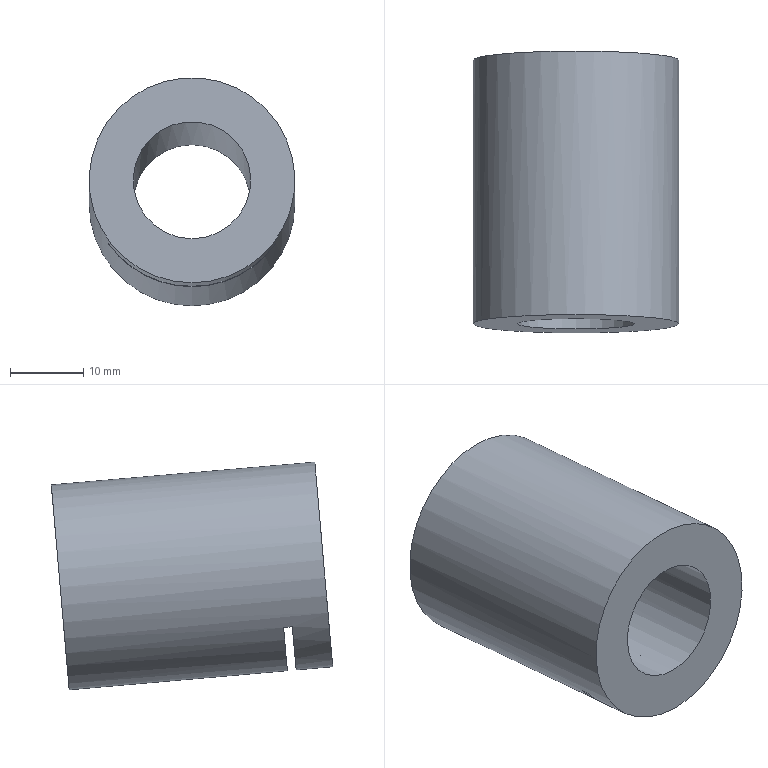Part | NX | features solid 2 | 1 solid | 7 faces | box 28 x 38.303 x 31.031 mm | volume 14816 mm3 | plane 5 | cylinder 2 | commonest cylinder face diameters 16 x1 28 x1
STEP:
#1=CARTESIAN_POINT('',(-120.452,-63.958,-21.398));
#2=VERTEX_POINT('',#1);
#3=CARTESIAN_POINT('',(-120.452,-65.178,-35.345));
#4=DIRECTION('',(0.,0.9962,-0.08716));
#5=DIRECTION('',(0.,0.08716,0.9962));
#6=AXIS2_PLACEMENT_3D('',#3,#4,#5);
#7=CIRCLE('',#6,14.);
#8=EDGE_CURVE('',#2,#2,#7,.F.);
#9=ORIENTED_EDGE('',*,*,#8,.T.);
#10=EDGE_LOOP('',(#9));
#11=FACE_BOUND('',#10,.T.);
#12=CARTESIAN_POINT('',(-120.452,-102.261,-46.154));
#13=VERTEX_POINT('',#12);
#14=CARTESIAN_POINT('',(-120.452,-101.041,-32.207));
#15=DIRECTION('',(0.,-0.9962,0.08716));
#16=DIRECTION('',(0.,-0.08716,-0.9962));
#17=AXIS2_PLACEMENT_3D('',#14,#15,#16);
#18=CIRCLE('',#17,14.);
#19=EDGE_CURVE('',#13,#13,#18,.T.);
#20=ORIENTED_EDGE('',*,*,#19,.F.);
#21=EDGE_LOOP('',(#20));
#22=FACE_BOUND('',#21,.T.);
#23=CARTESIAN_POINT('',(-109.034,-96.766,-40.712));
#24=VERTEX_POINT('',#23);
#25=CARTESIAN_POINT('',(-109.034,-95.571,-40.817));
#26=VERTEX_POINT('',#25);
#27=CARTESIAN_POINT('',(-109.034,-59.907,-43.937));
#28=DIRECTION('',(0.,-0.9962,0.08716));
#29=VECTOR('',#28,1000.);
#30=LINE('',#27,#29);
#31=EDGE_CURVE('',#24,#26,#30,.F.);
#32=ORIENTED_EDGE('',*,*,#31,.T.);
#33=CARTESIAN_POINT('',(-131.871,-95.571,-40.817));
#34=VERTEX_POINT('',#33);
#35=CARTESIAN_POINT('',(-120.452,-94.865,-32.748));
#36=DIRECTION('',(0.,-0.9962,0.08716));
#37=DIRECTION('',(0.,-0.08716,-0.9962));
#38=AXIS2_PLACEMENT_3D('',#35,#36,#37);
#39=CIRCLE('',#38,14.);
#40=EDGE_CURVE('',#26,#34,#39,.F.);
#41=ORIENTED_EDGE('',*,*,#40,.T.);
#42=CARTESIAN_POINT('',(-131.871,-96.766,-40.712));
#43=VERTEX_POINT('',#42);
#44=CARTESIAN_POINT('',(-131.871,-59.907,-43.937));
#45=DIRECTION('',(0.,-0.9962,0.08716));
#46=VECTOR('',#45,1000.);
#47=LINE('',#44,#46);
#48=EDGE_CURVE('',#34,#43,#47,.T.);
#49=ORIENTED_EDGE('',*,*,#48,.T.);
#50=CARTESIAN_POINT('',(-120.452,-96.06,-32.643));
#51=DIRECTION('',(0.,-0.9962,0.08716));
#52=DIRECTION('',(0.,-0.08716,-0.9962));
#53=AXIS2_PLACEMENT_3D('',#50,#51,#52);
#54=CIRCLE('',#53,14.);
#55=EDGE_CURVE('',#24,#43,#54,.F.);
#56=ORIENTED_EDGE('',*,*,#55,.F.);
#57=EDGE_LOOP('',(#32,#41,#49,#56));
#58=FACE_BOUND('',#57,.T.);
#59=CARTESIAN_POINT('',(-120.452,-67.37,-35.153));
#60=DIRECTION('',(0.,-0.9962,0.08716));
#61=DIRECTION('',(0.,-0.08716,-0.9962));
#62=AXIS2_PLACEMENT_3D('',#59,#60,#61);
#63=CYLINDRICAL_SURFACE('',#62,14.);
#64=ADVANCED_FACE('',(#11,#22,#58),#63,.T.);
#65=CARTESIAN_POINT('',(-120.452,-101.738,-40.177));
#66=VERTEX_POINT('',#65);
#67=CARTESIAN_POINT('',(-120.452,-101.041,-32.207));
#68=DIRECTION('',(0.,-0.9962,0.08716));
#69=DIRECTION('',(0.,-0.08716,-0.9962));
#70=AXIS2_PLACEMENT_3D('',#67,#68,#69);
#71=CIRCLE('',#70,8.);
#72=EDGE_CURVE('',#66,#66,#71,.T.);
#73=ORIENTED_EDGE('',*,*,#72,.F.);
#74=EDGE_LOOP('',(#73));
#75=FACE_BOUND('',#74,.T.);
#76=ORIENTED_EDGE('',*,*,#19,.T.);
#77=EDGE_LOOP('',(#76));
#78=FACE_BOUND('',#77,.T.);
#79=CARTESIAN_POINT('',(-120.452,-101.041,-32.207));
#80=DIRECTION('',(0.,-0.9962,0.08716));
#81=DIRECTION('',(-1.,0.,0.));
#82=AXIS2_PLACEMENT_3D('',#79,#80,#81);
#83=PLANE('',#82);
#84=ADVANCED_FACE('',(#75,#78),#83,.T.);
#85=CARTESIAN_POINT('',(-120.452,-64.481,-27.375));
#86=VERTEX_POINT('',#85);
#87=CARTESIAN_POINT('',(-120.452,-65.178,-35.345));
#88=DIRECTION('',(0.,0.9962,-0.08716));
#89=DIRECTION('',(0.,0.08716,0.9962));
#90=AXIS2_PLACEMENT_3D('',#87,#88,#89);
#91=CIRCLE('',#90,8.);
#92=EDGE_CURVE('',#86,#86,#91,.F.);
#93=ORIENTED_EDGE('',*,*,#92,.T.);
#94=EDGE_LOOP('',(#93));
#95=FACE_BOUND('',#94,.T.);
#96=ORIENTED_EDGE('',*,*,#8,.F.);
#97=EDGE_LOOP('',(#96));
#98=FACE_BOUND('',#97,.T.);
#99=CARTESIAN_POINT('',(-120.452,-65.178,-35.345));
#100=DIRECTION('',(0.,0.9962,-0.08716));
#101=DIRECTION('',(-1.,0.,0.));
#102=AXIS2_PLACEMENT_3D('',#99,#100,#101);
#103=PLANE('',#102);
#104=ADVANCED_FACE('',(#95,#98),#103,.T.);
#105=ORIENTED_EDGE('',*,*,#72,.T.);
#106=EDGE_LOOP('',(#105));
#107=FACE_BOUND('',#106,.T.);
#108=ORIENTED_EDGE('',*,*,#92,.F.);
#109=EDGE_LOOP('',(#108));
#110=FACE_BOUND('',#109,.T.);
#111=CARTESIAN_POINT('',(-120.452,-65.377,-35.327));
#112=DIRECTION('',(0.,-0.9962,0.08716));
#113=DIRECTION('',(0.,-0.08716,-0.9962));
#114=AXIS2_PLACEMENT_3D('',#111,#112,#113);
#115=CYLINDRICAL_SURFACE('',#114,8.);
#116=ADVANCED_FACE('',(#107,#110),#115,.F.);
#117=CARTESIAN_POINT('',(-131.942,-95.571,-40.817));
#118=DIRECTION('',(-1.,0.,0.));
#119=VECTOR('',#118,1000.);
#120=LINE('',#117,#119);
#121=EDGE_CURVE('',#34,#26,#120,.F.);
#122=ORIENTED_EDGE('',*,*,#121,.F.);
#123=ORIENTED_EDGE('',*,*,#40,.F.);
#124=EDGE_LOOP('',(#122,#123));
#125=FACE_BOUND('',#124,.T.);
#126=CARTESIAN_POINT('',(-131.942,-99.929,-90.626));
#127=DIRECTION('',(0.,-0.9962,0.08716));
#128=DIRECTION('',(0.,-0.08716,-0.9962));
#129=AXIS2_PLACEMENT_3D('',#126,#127,#128);
#130=PLANE('',#129);
#131=ADVANCED_FACE('',(#125),#130,.T.);
#132=ORIENTED_EDGE('',*,*,#55,.T.);
#133=CARTESIAN_POINT('',(-131.942,-96.766,-40.712));
#134=DIRECTION('',(-1.,0.,0.));
#135=VECTOR('',#134,1000.);
#136=LINE('',#133,#135);
#137=EDGE_CURVE('',#43,#24,#136,.F.);
#138=ORIENTED_EDGE('',*,*,#137,.T.);
#139=EDGE_LOOP('',(#132,#138));
#140=FACE_BOUND('',#139,.T.);
#141=CARTESIAN_POINT('',(-131.942,-101.124,-90.522));
#142=DIRECTION('',(0.,-0.9962,0.08716));
#143=DIRECTION('',(0.,-0.08716,-0.9962));
#144=AXIS2_PLACEMENT_3D('',#141,#142,#143);
#145=PLANE('',#144);
#146=ADVANCED_FACE('',(#140),#145,.F.);
#147=ORIENTED_EDGE('',*,*,#121,.T.);
#148=ORIENTED_EDGE('',*,*,#31,.F.);
#149=ORIENTED_EDGE('',*,*,#137,.F.);
#150=ORIENTED_EDGE('',*,*,#48,.F.);
#151=EDGE_LOOP('',(#147,#148,#149,#150));
#152=FACE_BOUND('',#151,.T.);
#153=CARTESIAN_POINT('',(-131.942,-96.766,-40.712));
#154=DIRECTION('',(0.,0.08716,0.9962));
#155=DIRECTION('',(0.,0.9962,-0.08716));
#156=AXIS2_PLACEMENT_3D('',#153,#154,#155);
#157=PLANE('',#156);
#158=ADVANCED_FACE('',(#152),#157,.F.);
#159=CLOSED_SHELL('',(#64,#84,#104,#116,#131,#146,#158));
#160=MANIFOLD_SOLID_BREP('',#159);
#161=(LENGTH_UNIT()NAMED_UNIT(*)SI_UNIT(.MILLI.,.METRE.));
#162=UNCERTAINTY_MEASURE_WITH_UNIT(LENGTH_MEASURE(0.00001),#161,'','');
#163=(NAMED_UNIT(*)PLANE_ANGLE_UNIT()SI_UNIT($,.RADIAN.));
#164=(NAMED_UNIT(*)SI_UNIT($,.STERADIAN.)SOLID_ANGLE_UNIT());
#165=(GEOMETRIC_REPRESENTATION_CONTEXT(3)GLOBAL_UNCERTAINTY_ASSIGNED_CONTEXT((#162))GLOBAL_UNIT_ASSIGNED_CONTEXT((#161,#163,#164))REPRESENTATION_CONTEXT('',''));
#166=ADVANCED_BREP_SHAPE_REPRESENTATION('',(#160),#165);